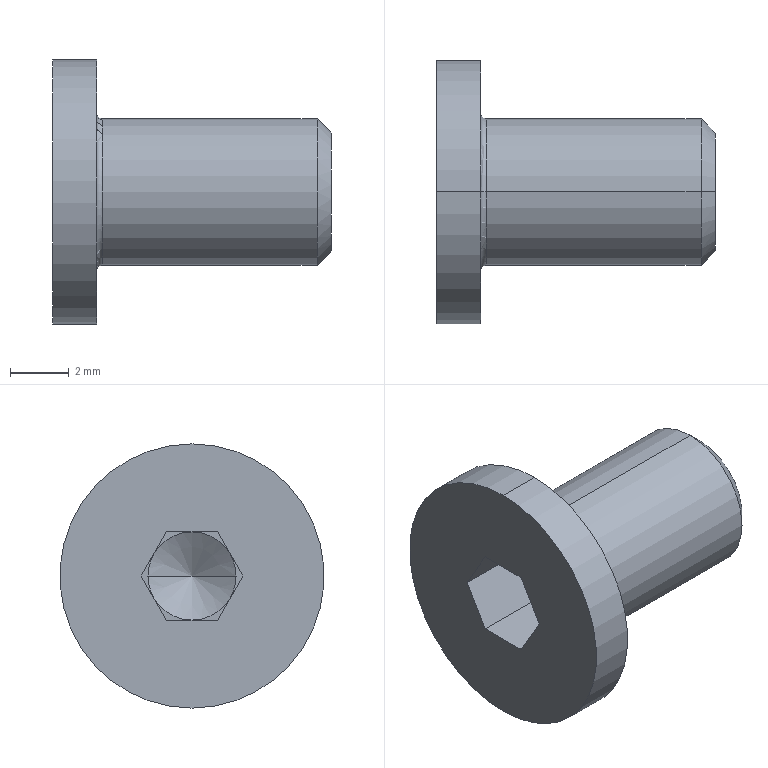Part | STEP file | CBSTS5-8-1 | 1 solid | 25 faces | box 9.5 x 9 x 9 mm | volume 225.454 mm3 | plane 15 | cone 4 | cylinder 4 | torus 2 | commonest cylinder face diameters 5 x2 9 x2
STEP:
#1=CARTESIAN_POINT('',(2.366,0.,0.));
#2=VERTEX_POINT('',#1);
#3=CARTESIAN_POINT('',(1.5,-1.5,0.));
#4=VERTEX_POINT('',#3);
#5=CARTESIAN_POINT('',(1.5,-1.5,0.));
#6=DIRECTION('',(-0.5,-0.866,0.));
#7=VECTOR('',#6,1000.);
#8=LINE('',#5,#7);
#9=EDGE_CURVE('',#2,#4,#8,.T.);
#10=ORIENTED_EDGE('',*,*,#9,.F.);
#11=CARTESIAN_POINT('',(1.5,1.5,0.));
#12=VERTEX_POINT('',#11);
#13=CARTESIAN_POINT('',(1.5,1.5,0.));
#14=DIRECTION('',(-0.5,0.866,0.));
#15=VECTOR('',#14,1000.);
#16=LINE('',#13,#15);
#17=EDGE_CURVE('',#2,#12,#16,.T.);
#18=ORIENTED_EDGE('',*,*,#17,.T.);
#19=CARTESIAN_POINT('',(1.5,1.299,-0.75));
#20=VERTEX_POINT('',#19);
#21=CARTESIAN_POINT('',(1.5,0.,0.));
#22=DIRECTION('',(1.,0.,0.));
#23=DIRECTION('',(0.,1.,0.));
#24=AXIS2_PLACEMENT_3D('',#21,#22,#23);
#25=CIRCLE('',#24,1.5);
#26=EDGE_CURVE('',#20,#12,#25,.T.);
#27=ORIENTED_EDGE('',*,*,#26,.F.);
#28=CARTESIAN_POINT('',(1.5,0.,-1.5));
#29=VERTEX_POINT('',#28);
#30=CARTESIAN_POINT('',(1.5,0.,0.));
#31=DIRECTION('',(1.,0.,0.));
#32=DIRECTION('',(0.,1.,0.));
#33=AXIS2_PLACEMENT_3D('',#30,#31,#32);
#34=CIRCLE('',#33,1.5);
#35=EDGE_CURVE('',#29,#20,#34,.T.);
#36=ORIENTED_EDGE('',*,*,#35,.F.);
#37=CARTESIAN_POINT('',(1.5,-1.299,-0.75));
#38=VERTEX_POINT('',#37);
#39=CARTESIAN_POINT('',(1.5,0.,0.));
#40=DIRECTION('',(1.,0.,0.));
#41=DIRECTION('',(0.,1.,0.));
#42=AXIS2_PLACEMENT_3D('',#39,#40,#41);
#43=CIRCLE('',#42,1.5);
#44=EDGE_CURVE('',#38,#29,#43,.T.);
#45=ORIENTED_EDGE('',*,*,#44,.F.);
#46=CARTESIAN_POINT('',(1.5,0.,0.));
#47=DIRECTION('',(1.,0.,0.));
#48=DIRECTION('',(0.,1.,0.));
#49=AXIS2_PLACEMENT_3D('',#46,#47,#48);
#50=CIRCLE('',#49,1.5);
#51=EDGE_CURVE('',#4,#38,#50,.T.);
#52=ORIENTED_EDGE('',*,*,#51,.F.);
#53=EDGE_LOOP('',(#10,#18,#27,#36,#45,#52));
#54=FACE_OUTER_BOUND('',#53,.T.);
#55=CARTESIAN_POINT('',(1.5,0.,0.));
#56=DIRECTION('',(-1.,0.,0.));
#57=DIRECTION('',(0.,-1.,0.));
#58=AXIS2_PLACEMENT_3D('',#55,#56,#57);
#59=CONICAL_SURFACE('',#58,1.5,1.047);
#60=ADVANCED_FACE('',(#54),#59,.F.);
#61=CARTESIAN_POINT('',(8.,0.,-2.01));
#62=VERTEX_POINT('',#61);
#63=CARTESIAN_POINT('',(8.,0.,2.01));
#64=VERTEX_POINT('',#63);
#65=CARTESIAN_POINT('',(8.,0.,0.));
#66=DIRECTION('',(1.,0.,0.));
#67=DIRECTION('',(0.,0.,-1.));
#68=AXIS2_PLACEMENT_3D('',#65,#66,#67);
#69=CIRCLE('',#68,2.01);
#70=EDGE_CURVE('',#62,#64,#69,.T.);
#71=ORIENTED_EDGE('',*,*,#70,.F.);
#72=CARTESIAN_POINT('',(7.51,0.,-2.5));
#73=VERTEX_POINT('',#72);
#74=CARTESIAN_POINT('',(7.51,0.,-2.5));
#75=DIRECTION('',(-0.7071,0.,-0.7071));
#76=VECTOR('',#75,1000.);
#77=LINE('',#74,#76);
#78=EDGE_CURVE('',#62,#73,#77,.T.);
#79=ORIENTED_EDGE('',*,*,#78,.T.);
#80=CARTESIAN_POINT('',(7.51,0.,2.5));
#81=VERTEX_POINT('',#80);
#82=CARTESIAN_POINT('',(7.51,0.,0.));
#83=DIRECTION('',(1.,0.,0.));
#84=DIRECTION('',(0.,0.,-1.));
#85=AXIS2_PLACEMENT_3D('',#82,#83,#84);
#86=CIRCLE('',#85,2.5);
#87=EDGE_CURVE('',#73,#81,#86,.T.);
#88=ORIENTED_EDGE('',*,*,#87,.T.);
#89=CARTESIAN_POINT('',(7.51,0.,2.5));
#90=DIRECTION('',(-0.7071,0.,0.7071));
#91=VECTOR('',#90,1000.);
#92=LINE('',#89,#91);
#93=EDGE_CURVE('',#64,#81,#92,.T.);
#94=ORIENTED_EDGE('',*,*,#93,.F.);
#95=EDGE_LOOP('',(#71,#79,#88,#94));
#96=FACE_OUTER_BOUND('',#95,.T.);
#97=CARTESIAN_POINT('',(7.51,0.,0.));
#98=DIRECTION('',(-1.,0.,0.));
#99=DIRECTION('',(0.,0.,1.));
#100=AXIS2_PLACEMENT_3D('',#97,#98,#99);
#101=CONICAL_SURFACE('',#100,2.5,0.7854);
#102=ADVANCED_FACE('',(#96),#101,.T.);
#103=CARTESIAN_POINT('',(0.2,0.,-2.5));
#104=VERTEX_POINT('',#103);
#105=CARTESIAN_POINT('',(0.2,0.,2.5));
#106=VERTEX_POINT('',#105);
#107=CARTESIAN_POINT('',(0.2,0.,0.));
#108=DIRECTION('',(1.,0.,0.));
#109=DIRECTION('',(0.,0.,-1.));
#110=AXIS2_PLACEMENT_3D('',#107,#108,#109);
#111=CIRCLE('',#110,2.5);
#112=EDGE_CURVE('',#104,#106,#111,.T.);
#113=ORIENTED_EDGE('',*,*,#112,.T.);
#114=CARTESIAN_POINT('',(8.,0.,2.5));
#115=DIRECTION('',(1.,0.,0.));
#116=VECTOR('',#115,1000.);
#117=LINE('',#114,#116);
#118=EDGE_CURVE('',#106,#81,#117,.T.);
#119=ORIENTED_EDGE('',*,*,#118,.T.);
#120=ORIENTED_EDGE('',*,*,#87,.F.);
#121=CARTESIAN_POINT('',(8.,0.,-2.5));
#122=DIRECTION('',(1.,0.,0.));
#123=VECTOR('',#122,1000.);
#124=LINE('',#121,#123);
#125=EDGE_CURVE('',#104,#73,#124,.T.);
#126=ORIENTED_EDGE('',*,*,#125,.F.);
#127=EDGE_LOOP('',(#113,#119,#120,#126));
#128=FACE_OUTER_BOUND('',#127,.T.);
#129=CARTESIAN_POINT('',(8.,0.,0.));
#130=DIRECTION('',(1.,0.,0.));
#131=DIRECTION('',(0.,0.,-1.));
#132=AXIS2_PLACEMENT_3D('',#129,#130,#131);
#133=CYLINDRICAL_SURFACE('',#132,2.5);
#134=ADVANCED_FACE('',(#128),#133,.T.);
#135=CARTESIAN_POINT('',(0.2,0.,0.));
#136=DIRECTION('',(1.,0.,0.));
#137=DIRECTION('',(0.,0.,-1.));
#138=AXIS2_PLACEMENT_3D('',#135,#136,#137);
#139=CIRCLE('',#138,2.5);
#140=EDGE_CURVE('',#106,#104,#139,.T.);
#141=ORIENTED_EDGE('',*,*,#140,.F.);
#142=CARTESIAN_POINT('',(0.,0.,2.7));
#143=VERTEX_POINT('',#142);
#144=CARTESIAN_POINT('',(0.2,0.,2.7));
#145=DIRECTION('',(0.,1.,0.));
#146=DIRECTION('',(0.,0.,1.));
#147=AXIS2_PLACEMENT_3D('',#144,#145,#146);
#148=CIRCLE('',#147,0.2);
#149=EDGE_CURVE('',#106,#143,#148,.T.);
#150=ORIENTED_EDGE('',*,*,#149,.T.);
#151=CARTESIAN_POINT('',(0.,0.,-2.7));
#152=VERTEX_POINT('',#151);
#153=CARTESIAN_POINT('',(0.,0.,0.));
#154=DIRECTION('',(1.,0.,0.));
#155=DIRECTION('',(0.,0.,-1.));
#156=AXIS2_PLACEMENT_3D('',#153,#154,#155);
#157=CIRCLE('',#156,2.7);
#158=EDGE_CURVE('',#143,#152,#157,.T.);
#159=ORIENTED_EDGE('',*,*,#158,.T.);
#160=CARTESIAN_POINT('',(0.2,0.,-2.7));
#161=DIRECTION('',(0.,-1.,0.));
#162=DIRECTION('',(0.,0.,-1.));
#163=AXIS2_PLACEMENT_3D('',#160,#161,#162);
#164=CIRCLE('',#163,0.2);
#165=EDGE_CURVE('',#104,#152,#164,.T.);
#166=ORIENTED_EDGE('',*,*,#165,.F.);
#167=EDGE_LOOP('',(#141,#150,#159,#166));
#168=FACE_OUTER_BOUND('',#167,.T.);
#169=CARTESIAN_POINT('',(0.2,0.,0.));
#170=DIRECTION('',(1.,0.,0.));
#171=DIRECTION('',(0.,0.,-1.));
#172=AXIS2_PLACEMENT_3D('',#169,#170,#171);
#173=TOROIDAL_SURFACE('',#172,2.7,0.2);
#174=ADVANCED_FACE('',(#168),#173,.F.);
#175=CARTESIAN_POINT('',(-1.5,0.,-4.5));
#176=VERTEX_POINT('',#175);
#177=CARTESIAN_POINT('',(-1.5,0.,4.5));
#178=VERTEX_POINT('',#177);
#179=CARTESIAN_POINT('',(-1.5,0.,0.));
#180=DIRECTION('',(1.,0.,0.));
#181=DIRECTION('',(0.,0.,-1.));
#182=AXIS2_PLACEMENT_3D('',#179,#180,#181);
#183=CIRCLE('',#182,4.5);
#184=EDGE_CURVE('',#176,#178,#183,.T.);
#185=ORIENTED_EDGE('',*,*,#184,.T.);
#186=CARTESIAN_POINT('',(0.,0.,4.5));
#187=VERTEX_POINT('',#186);
#188=CARTESIAN_POINT('',(8.,0.,4.5));
#189=DIRECTION('',(1.,0.,0.));
#190=VECTOR('',#189,1000.);
#191=LINE('',#188,#190);
#192=EDGE_CURVE('',#178,#187,#191,.T.);
#193=ORIENTED_EDGE('',*,*,#192,.T.);
#194=CARTESIAN_POINT('',(0.,0.,-4.5));
#195=VERTEX_POINT('',#194);
#196=CARTESIAN_POINT('',(0.,0.,0.));
#197=DIRECTION('',(1.,0.,0.));
#198=DIRECTION('',(0.,0.,-1.));
#199=AXIS2_PLACEMENT_3D('',#196,#197,#198);
#200=CIRCLE('',#199,4.5);
#201=EDGE_CURVE('',#195,#187,#200,.T.);
#202=ORIENTED_EDGE('',*,*,#201,.F.);
#203=CARTESIAN_POINT('',(8.,0.,-4.5));
#204=DIRECTION('',(1.,0.,0.));
#205=VECTOR('',#204,1000.);
#206=LINE('',#203,#205);
#207=EDGE_CURVE('',#176,#195,#206,.T.);
#208=ORIENTED_EDGE('',*,*,#207,.F.);
#209=EDGE_LOOP('',(#185,#193,#202,#208));
#210=FACE_OUTER_BOUND('',#209,.T.);
#211=CARTESIAN_POINT('',(8.,0.,0.));
#212=DIRECTION('',(1.,0.,0.));
#213=DIRECTION('',(0.,0.,-1.));
#214=AXIS2_PLACEMENT_3D('',#211,#212,#213);
#215=CYLINDRICAL_SURFACE('',#214,4.5);
#216=ADVANCED_FACE('',(#210),#215,.T.);
#217=ORIENTED_EDGE('',*,*,#184,.F.);
#218=CARTESIAN_POINT('',(-1.5,0.,0.));
#219=DIRECTION('',(1.,0.,0.));
#220=DIRECTION('',(0.,0.,-1.));
#221=AXIS2_PLACEMENT_3D('',#218,#219,#220);
#222=CIRCLE('',#221,4.5);
#223=EDGE_CURVE('',#178,#176,#222,.T.);
#224=ORIENTED_EDGE('',*,*,#223,.F.);
#225=EDGE_LOOP('',(#217,#224));
#226=FACE_OUTER_BOUND('',#225,.T.);
#227=CARTESIAN_POINT('',(-1.5,-1.732,0.));
#228=VERTEX_POINT('',#227);
#229=CARTESIAN_POINT('',(-1.5,-0.866,-1.5));
#230=VERTEX_POINT('',#229);
#231=CARTESIAN_POINT('',(-1.5,-1.732,0.));
#232=DIRECTION('',(0.,0.5,-0.866));
#233=VECTOR('',#232,1000.);
#234=LINE('',#231,#233);
#235=EDGE_CURVE('',#228,#230,#234,.T.);
#236=ORIENTED_EDGE('',*,*,#235,.T.);
#237=CARTESIAN_POINT('',(-1.5,0.866,-1.5));
#238=VERTEX_POINT('',#237);
#239=CARTESIAN_POINT('',(-1.5,-0.866,-1.5));
#240=DIRECTION('',(0.,1.,0.));
#241=VECTOR('',#240,1000.);
#242=LINE('',#239,#241);
#243=EDGE_CURVE('',#230,#238,#242,.T.);
#244=ORIENTED_EDGE('',*,*,#243,.T.);
#245=CARTESIAN_POINT('',(-1.5,1.732,0.));
#246=VERTEX_POINT('',#245);
#247=CARTESIAN_POINT('',(-1.5,0.866,-1.5));
#248=DIRECTION('',(0.,0.5,0.866));
#249=VECTOR('',#248,1000.);
#250=LINE('',#247,#249);
#251=EDGE_CURVE('',#238,#246,#250,.T.);
#252=ORIENTED_EDGE('',*,*,#251,.T.);
#253=CARTESIAN_POINT('',(-1.5,0.866,1.5));
#254=VERTEX_POINT('',#253);
#255=CARTESIAN_POINT('',(-1.5,1.732,0.));
#256=DIRECTION('',(0.,-0.5,0.866));
#257=VECTOR('',#256,1000.);
#258=LINE('',#255,#257);
#259=EDGE_CURVE('',#246,#254,#258,.T.);
#260=ORIENTED_EDGE('',*,*,#259,.T.);
#261=CARTESIAN_POINT('',(-1.5,-0.866,1.5));
#262=VERTEX_POINT('',#261);
#263=CARTESIAN_POINT('',(-1.5,0.866,1.5));
#264=DIRECTION('',(0.,-1.,0.));
#265=VECTOR('',#264,1000.);
#266=LINE('',#263,#265);
#267=EDGE_CURVE('',#254,#262,#266,.T.);
#268=ORIENTED_EDGE('',*,*,#267,.T.);
#269=CARTESIAN_POINT('',(-1.5,-0.866,1.5));
#270=DIRECTION('',(0.,-0.5,-0.866));
#271=VECTOR('',#270,1000.);
#272=LINE('',#269,#271);
#273=EDGE_CURVE('',#262,#228,#272,.T.);
#274=ORIENTED_EDGE('',*,*,#273,.T.);
#275=EDGE_LOOP('',(#236,#244,#252,#260,#268,#274));
#276=FACE_BOUND('',#275,.T.);
#277=CARTESIAN_POINT('',(-1.5,0.,0.));
#278=DIRECTION('',(1.,0.,0.));
#279=DIRECTION('',(0.,0.,-1.));
#280=AXIS2_PLACEMENT_3D('',#277,#278,#279);
#281=PLANE('',#280);
#282=ADVANCED_FACE('',(#226,#276),#281,.F.);
#283=ORIENTED_EDGE('',*,*,#192,.F.);
#284=ORIENTED_EDGE('',*,*,#223,.T.);
#285=ORIENTED_EDGE('',*,*,#207,.T.);
#286=CARTESIAN_POINT('',(0.,0.,0.));
#287=DIRECTION('',(1.,0.,0.));
#288=DIRECTION('',(0.,0.,-1.));
#289=AXIS2_PLACEMENT_3D('',#286,#287,#288);
#290=CIRCLE('',#289,4.5);
#291=EDGE_CURVE('',#187,#195,#290,.T.);
#292=ORIENTED_EDGE('',*,*,#291,.F.);
#293=EDGE_LOOP('',(#283,#284,#285,#292));
#294=FACE_OUTER_BOUND('',#293,.T.);
#295=CARTESIAN_POINT('',(8.,0.,0.));
#296=DIRECTION('',(1.,0.,0.));
#297=DIRECTION('',(0.,0.,-1.));
#298=AXIS2_PLACEMENT_3D('',#295,#296,#297);
#299=CYLINDRICAL_SURFACE('',#298,4.5);
#300=ADVANCED_FACE('',(#294),#299,.T.);
#301=CARTESIAN_POINT('',(0.,0.,0.));
#302=DIRECTION('',(1.,0.,0.));
#303=DIRECTION('',(0.,0.,-1.));
#304=AXIS2_PLACEMENT_3D('',#301,#302,#303);
#305=CIRCLE('',#304,2.7);
#306=EDGE_CURVE('',#152,#143,#305,.T.);
#307=ORIENTED_EDGE('',*,*,#306,.F.);
#308=ORIENTED_EDGE('',*,*,#158,.F.);
#309=EDGE_LOOP('',(#307,#308));
#310=FACE_BOUND('',#309,.T.);
#311=ORIENTED_EDGE('',*,*,#201,.T.);
#312=ORIENTED_EDGE('',*,*,#291,.T.);
#313=EDGE_LOOP('',(#311,#312));
#314=FACE_OUTER_BOUND('',#313,.T.);
#315=CARTESIAN_POINT('',(0.,4.5,0.));
#316=DIRECTION('',(-1.,0.,0.));
#317=DIRECTION('',(0.,0.,1.));
#318=AXIS2_PLACEMENT_3D('',#315,#316,#317);
#319=PLANE('',#318);
#320=ADVANCED_FACE('',(#310,#314),#319,.F.);
#321=ORIENTED_EDGE('',*,*,#149,.F.);
#322=ORIENTED_EDGE('',*,*,#112,.F.);
#323=ORIENTED_EDGE('',*,*,#165,.T.);
#324=ORIENTED_EDGE('',*,*,#306,.T.);
#325=EDGE_LOOP('',(#321,#322,#323,#324));
#326=FACE_OUTER_BOUND('',#325,.T.);
#327=CARTESIAN_POINT('',(0.2,0.,0.));
#328=DIRECTION('',(1.,0.,0.));
#329=DIRECTION('',(0.,0.,-1.));
#330=AXIS2_PLACEMENT_3D('',#327,#328,#329);
#331=TOROIDAL_SURFACE('',#330,2.7,0.2);
#332=ADVANCED_FACE('',(#326),#331,.F.);
#333=ORIENTED_EDGE('',*,*,#118,.F.);
#334=ORIENTED_EDGE('',*,*,#140,.T.);
#335=ORIENTED_EDGE('',*,*,#125,.T.);
#336=CARTESIAN_POINT('',(7.51,0.,0.));
#337=DIRECTION('',(1.,0.,0.));
#338=DIRECTION('',(0.,0.,-1.));
#339=AXIS2_PLACEMENT_3D('',#336,#337,#338);
#340=CIRCLE('',#339,2.5);
#341=EDGE_CURVE('',#81,#73,#340,.T.);
#342=ORIENTED_EDGE('',*,*,#341,.F.);
#343=EDGE_LOOP('',(#333,#334,#335,#342));
#344=FACE_OUTER_BOUND('',#343,.T.);
#345=CARTESIAN_POINT('',(8.,0.,0.));
#346=DIRECTION('',(1.,0.,0.));
#347=DIRECTION('',(0.,0.,-1.));
#348=AXIS2_PLACEMENT_3D('',#345,#346,#347);
#349=CYLINDRICAL_SURFACE('',#348,2.5);
#350=ADVANCED_FACE('',(#344),#349,.T.);
#351=ORIENTED_EDGE('',*,*,#78,.F.);
#352=CARTESIAN_POINT('',(8.,0.,0.));
#353=DIRECTION('',(1.,0.,0.));
#354=DIRECTION('',(0.,0.,-1.));
#355=AXIS2_PLACEMENT_3D('',#352,#353,#354);
#356=CIRCLE('',#355,2.01);
#357=EDGE_CURVE('',#64,#62,#356,.T.);
#358=ORIENTED_EDGE('',*,*,#357,.F.);
#359=ORIENTED_EDGE('',*,*,#93,.T.);
#360=ORIENTED_EDGE('',*,*,#341,.T.);
#361=EDGE_LOOP('',(#351,#358,#359,#360));
#362=FACE_OUTER_BOUND('',#361,.T.);
#363=CARTESIAN_POINT('',(7.51,0.,0.));
#364=DIRECTION('',(-1.,0.,0.));
#365=DIRECTION('',(0.,0.,1.));
#366=AXIS2_PLACEMENT_3D('',#363,#364,#365);
#367=CONICAL_SURFACE('',#366,2.5,0.7854);
#368=ADVANCED_FACE('',(#362),#367,.T.);
#369=ORIENTED_EDGE('',*,*,#357,.T.);
#370=ORIENTED_EDGE('',*,*,#70,.T.);
#371=EDGE_LOOP('',(#369,#370));
#372=FACE_OUTER_BOUND('',#371,.T.);
#373=CARTESIAN_POINT('',(8.,2.01,0.));
#374=DIRECTION('',(-1.,0.,0.));
#375=DIRECTION('',(0.,0.,1.));
#376=AXIS2_PLACEMENT_3D('',#373,#374,#375);
#377=PLANE('',#376);
#378=ADVANCED_FACE('',(#372),#377,.F.);
#379=ORIENTED_EDGE('',*,*,#267,.F.);
#380=CARTESIAN_POINT('',(1.5,0.866,1.5));
#381=VERTEX_POINT('',#380);
#382=CARTESIAN_POINT('',(1.5,0.866,1.5));
#383=DIRECTION('',(-1.,0.,0.));
#384=VECTOR('',#383,1000.);
#385=LINE('',#382,#384);
#386=EDGE_CURVE('',#381,#254,#385,.T.);
#387=ORIENTED_EDGE('',*,*,#386,.F.);
#388=CARTESIAN_POINT('',(1.5,0.,1.5));
#389=VERTEX_POINT('',#388);
#390=CARTESIAN_POINT('',(1.5,0.866,1.5));
#391=DIRECTION('',(0.,-1.,0.));
#392=VECTOR('',#391,1000.);
#393=LINE('',#390,#392);
#394=EDGE_CURVE('',#381,#389,#393,.T.);
#395=ORIENTED_EDGE('',*,*,#394,.T.);
#396=CARTESIAN_POINT('',(1.5,-0.866,1.5));
#397=VERTEX_POINT('',#396);
#398=CARTESIAN_POINT('',(1.5,0.866,1.5));
#399=DIRECTION('',(0.,-1.,0.));
#400=VECTOR('',#399,1000.);
#401=LINE('',#398,#400);
#402=EDGE_CURVE('',#389,#397,#401,.T.);
#403=ORIENTED_EDGE('',*,*,#402,.T.);
#404=CARTESIAN_POINT('',(1.5,-0.866,1.5));
#405=DIRECTION('',(-1.,0.,0.));
#406=VECTOR('',#405,1000.);
#407=LINE('',#404,#406);
#408=EDGE_CURVE('',#397,#262,#407,.T.);
#409=ORIENTED_EDGE('',*,*,#408,.T.);
#410=EDGE_LOOP('',(#379,#387,#395,#403,#409));
#411=FACE_OUTER_BOUND('',#410,.T.);
#412=CARTESIAN_POINT('',(1.5,0.866,1.5));
#413=DIRECTION('',(0.,0.,-1.));
#414=DIRECTION('',(-1.,0.,0.));
#415=AXIS2_PLACEMENT_3D('',#412,#413,#414);
#416=PLANE('',#415);
#417=ADVANCED_FACE('',(#411),#416,.T.);
#418=ORIENTED_EDGE('',*,*,#273,.F.);
#419=ORIENTED_EDGE('',*,*,#408,.F.);
#420=CARTESIAN_POINT('',(1.5,-1.299,0.75));
#421=VERTEX_POINT('',#420);
#422=CARTESIAN_POINT('',(1.5,-0.866,1.5));
#423=DIRECTION('',(0.,-0.5,-0.866));
#424=VECTOR('',#423,1000.);
#425=LINE('',#422,#424);
#426=EDGE_CURVE('',#397,#421,#425,.T.);
#427=ORIENTED_EDGE('',*,*,#426,.T.);
#428=CARTESIAN_POINT('',(1.5,-1.732,0.));
#429=VERTEX_POINT('',#428);
#430=CARTESIAN_POINT('',(1.5,-0.866,1.5));
#431=DIRECTION('',(0.,-0.5,-0.866));
#432=VECTOR('',#431,1000.);
#433=LINE('',#430,#432);
#434=EDGE_CURVE('',#421,#429,#433,.T.);
#435=ORIENTED_EDGE('',*,*,#434,.T.);
#436=CARTESIAN_POINT('',(1.5,-1.732,0.));
#437=DIRECTION('',(-1.,0.,0.));
#438=VECTOR('',#437,1000.);
#439=LINE('',#436,#438);
#440=EDGE_CURVE('',#429,#228,#439,.T.);
#441=ORIENTED_EDGE('',*,*,#440,.T.);
#442=EDGE_LOOP('',(#418,#419,#427,#435,#441));
#443=FACE_OUTER_BOUND('',#442,.T.);
#444=CARTESIAN_POINT('',(1.5,-0.866,1.5));
#445=DIRECTION('',(0.,0.866,-0.5));
#446=DIRECTION('',(0.,0.5,0.866));
#447=AXIS2_PLACEMENT_3D('',#444,#445,#446);
#448=PLANE('',#447);
#449=ADVANCED_FACE('',(#443),#448,.T.);
#450=ORIENTED_EDGE('',*,*,#235,.F.);
#451=ORIENTED_EDGE('',*,*,#440,.F.);
#452=CARTESIAN_POINT('',(1.5,-1.732,0.));
#453=DIRECTION('',(0.,0.5,-0.866));
#454=VECTOR('',#453,1000.);
#455=LINE('',#452,#454);
#456=EDGE_CURVE('',#429,#38,#455,.T.);
#457=ORIENTED_EDGE('',*,*,#456,.T.);
#458=CARTESIAN_POINT('',(1.5,-0.866,-1.5));
#459=VERTEX_POINT('',#458);
#460=CARTESIAN_POINT('',(1.5,-1.732,0.));
#461=DIRECTION('',(0.,0.5,-0.866));
#462=VECTOR('',#461,1000.);
#463=LINE('',#460,#462);
#464=EDGE_CURVE('',#38,#459,#463,.T.);
#465=ORIENTED_EDGE('',*,*,#464,.T.);
#466=CARTESIAN_POINT('',(1.5,-0.866,-1.5));
#467=DIRECTION('',(-1.,0.,0.));
#468=VECTOR('',#467,1000.);
#469=LINE('',#466,#468);
#470=EDGE_CURVE('',#459,#230,#469,.T.);
#471=ORIENTED_EDGE('',*,*,#470,.T.);
#472=EDGE_LOOP('',(#450,#451,#457,#465,#471));
#473=FACE_OUTER_BOUND('',#472,.T.);
#474=CARTESIAN_POINT('',(1.5,-1.732,0.));
#475=DIRECTION('',(0.,0.866,0.5));
#476=DIRECTION('',(0.,-0.5,0.866));
#477=AXIS2_PLACEMENT_3D('',#474,#475,#476);
#478=PLANE('',#477);
#479=ADVANCED_FACE('',(#473),#478,.T.);
#480=ORIENTED_EDGE('',*,*,#243,.F.);
#481=ORIENTED_EDGE('',*,*,#470,.F.);
#482=CARTESIAN_POINT('',(1.5,-0.866,-1.5));
#483=DIRECTION('',(0.,1.,0.));
#484=VECTOR('',#483,1000.);
#485=LINE('',#482,#484);
#486=EDGE_CURVE('',#459,#29,#485,.T.);
#487=ORIENTED_EDGE('',*,*,#486,.T.);
#488=CARTESIAN_POINT('',(1.5,0.866,-1.5));
#489=VERTEX_POINT('',#488);
#490=CARTESIAN_POINT('',(1.5,-0.866,-1.5));
#491=DIRECTION('',(0.,1.,0.));
#492=VECTOR('',#491,1000.);
#493=LINE('',#490,#492);
#494=EDGE_CURVE('',#29,#489,#493,.T.);
#495=ORIENTED_EDGE('',*,*,#494,.T.);
#496=CARTESIAN_POINT('',(1.5,0.866,-1.5));
#497=DIRECTION('',(-1.,0.,0.));
#498=VECTOR('',#497,1000.);
#499=LINE('',#496,#498);
#500=EDGE_CURVE('',#489,#238,#499,.T.);
#501=ORIENTED_EDGE('',*,*,#500,.T.);
#502=EDGE_LOOP('',(#480,#481,#487,#495,#501));
#503=FACE_OUTER_BOUND('',#502,.T.);
#504=CARTESIAN_POINT('',(1.5,-0.866,-1.5));
#505=DIRECTION('',(0.,0.,1.));
#506=DIRECTION('',(1.,0.,0.));
#507=AXIS2_PLACEMENT_3D('',#504,#505,#506);
#508=PLANE('',#507);
#509=ADVANCED_FACE('',(#503),#508,.T.);
#510=ORIENTED_EDGE('',*,*,#251,.F.);
#511=ORIENTED_EDGE('',*,*,#500,.F.);
#512=CARTESIAN_POINT('',(1.5,0.866,-1.5));
#513=DIRECTION('',(0.,0.5,0.866));
#514=VECTOR('',#513,1000.);
#515=LINE('',#512,#514);
#516=EDGE_CURVE('',#489,#20,#515,.T.);
#517=ORIENTED_EDGE('',*,*,#516,.T.);
#518=CARTESIAN_POINT('',(1.5,1.732,0.));
#519=VERTEX_POINT('',#518);
#520=CARTESIAN_POINT('',(1.5,0.866,-1.5));
#521=DIRECTION('',(0.,0.5,0.866));
#522=VECTOR('',#521,1000.);
#523=LINE('',#520,#522);
#524=EDGE_CURVE('',#20,#519,#523,.T.);
#525=ORIENTED_EDGE('',*,*,#524,.T.);
#526=CARTESIAN_POINT('',(1.5,1.732,0.));
#527=DIRECTION('',(-1.,0.,0.));
#528=VECTOR('',#527,1000.);
#529=LINE('',#526,#528);
#530=EDGE_CURVE('',#519,#246,#529,.T.);
#531=ORIENTED_EDGE('',*,*,#530,.T.);
#532=EDGE_LOOP('',(#510,#511,#517,#525,#531));
#533=FACE_OUTER_BOUND('',#532,.T.);
#534=CARTESIAN_POINT('',(1.5,0.866,-1.5));
#535=DIRECTION('',(0.,-0.866,0.5));
#536=DIRECTION('',(0.,-0.5,-0.866));
#537=AXIS2_PLACEMENT_3D('',#534,#535,#536);
#538=PLANE('',#537);
#539=ADVANCED_FACE('',(#533),#538,.T.);
#540=ORIENTED_EDGE('',*,*,#259,.F.);
#541=ORIENTED_EDGE('',*,*,#530,.F.);
#542=CARTESIAN_POINT('',(1.5,1.299,0.75));
#543=VERTEX_POINT('',#542);
#544=CARTESIAN_POINT('',(1.5,1.732,0.));
#545=DIRECTION('',(0.,-0.5,0.866));
#546=VECTOR('',#545,1000.);
#547=LINE('',#544,#546);
#548=EDGE_CURVE('',#519,#543,#547,.T.);
#549=ORIENTED_EDGE('',*,*,#548,.T.);
#550=CARTESIAN_POINT('',(1.5,1.732,0.));
#551=DIRECTION('',(0.,-0.5,0.866));
#552=VECTOR('',#551,1000.);
#553=LINE('',#550,#552);
#554=EDGE_CURVE('',#543,#381,#553,.T.);
#555=ORIENTED_EDGE('',*,*,#554,.T.);
#556=ORIENTED_EDGE('',*,*,#386,.T.);
#557=EDGE_LOOP('',(#540,#541,#549,#555,#556));
#558=FACE_OUTER_BOUND('',#557,.T.);
#559=CARTESIAN_POINT('',(1.5,1.732,0.));
#560=DIRECTION('',(0.,-0.866,-0.5));
#561=DIRECTION('',(0.,0.5,-0.866));
#562=AXIS2_PLACEMENT_3D('',#559,#560,#561);
#563=PLANE('',#562);
#564=ADVANCED_FACE('',(#558),#563,.T.);
#565=ORIENTED_EDGE('',*,*,#35,.T.);
#566=ORIENTED_EDGE('',*,*,#516,.F.);
#567=ORIENTED_EDGE('',*,*,#494,.F.);
#568=EDGE_LOOP('',(#565,#566,#567));
#569=FACE_OUTER_BOUND('',#568,.T.);
#570=CARTESIAN_POINT('',(1.5,0.,0.));
#571=DIRECTION('',(1.,0.,0.));
#572=DIRECTION('',(0.,0.,-1.));
#573=AXIS2_PLACEMENT_3D('',#570,#571,#572);
#574=PLANE('',#573);
#575=ADVANCED_FACE('',(#569),#574,.F.);
#576=ORIENTED_EDGE('',*,*,#524,.F.);
#577=ORIENTED_EDGE('',*,*,#26,.T.);
#578=CARTESIAN_POINT('',(1.5,0.,0.));
#579=DIRECTION('',(1.,0.,0.));
#580=DIRECTION('',(0.,1.,0.));
#581=AXIS2_PLACEMENT_3D('',#578,#579,#580);
#582=CIRCLE('',#581,1.5);
#583=EDGE_CURVE('',#12,#543,#582,.T.);
#584=ORIENTED_EDGE('',*,*,#583,.T.);
#585=ORIENTED_EDGE('',*,*,#548,.F.);
#586=EDGE_LOOP('',(#576,#577,#584,#585));
#587=FACE_OUTER_BOUND('',#586,.T.);
#588=CARTESIAN_POINT('',(1.5,0.,0.));
#589=DIRECTION('',(1.,0.,0.));
#590=DIRECTION('',(0.,0.,-1.));
#591=AXIS2_PLACEMENT_3D('',#588,#589,#590);
#592=PLANE('',#591);
#593=ADVANCED_FACE('',(#587),#592,.F.);
#594=CARTESIAN_POINT('',(1.5,0.,0.));
#595=DIRECTION('',(1.,0.,0.));
#596=DIRECTION('',(0.,1.,0.));
#597=AXIS2_PLACEMENT_3D('',#594,#595,#596);
#598=CIRCLE('',#597,1.5);
#599=EDGE_CURVE('',#543,#389,#598,.T.);
#600=ORIENTED_EDGE('',*,*,#599,.T.);
#601=ORIENTED_EDGE('',*,*,#394,.F.);
#602=ORIENTED_EDGE('',*,*,#554,.F.);
#603=EDGE_LOOP('',(#600,#601,#602));
#604=FACE_OUTER_BOUND('',#603,.T.);
#605=CARTESIAN_POINT('',(1.5,0.,0.));
#606=DIRECTION('',(1.,0.,0.));
#607=DIRECTION('',(0.,0.,-1.));
#608=AXIS2_PLACEMENT_3D('',#605,#606,#607);
#609=PLANE('',#608);
#610=ADVANCED_FACE('',(#604),#609,.F.);
#611=CARTESIAN_POINT('',(1.5,0.,0.));
#612=DIRECTION('',(1.,0.,0.));
#613=DIRECTION('',(0.,1.,0.));
#614=AXIS2_PLACEMENT_3D('',#611,#612,#613);
#615=CIRCLE('',#614,1.5);
#616=EDGE_CURVE('',#389,#421,#615,.T.);
#617=ORIENTED_EDGE('',*,*,#616,.T.);
#618=ORIENTED_EDGE('',*,*,#426,.F.);
#619=ORIENTED_EDGE('',*,*,#402,.F.);
#620=EDGE_LOOP('',(#617,#618,#619));
#621=FACE_OUTER_BOUND('',#620,.T.);
#622=CARTESIAN_POINT('',(1.5,0.,0.));
#623=DIRECTION('',(1.,0.,0.));
#624=DIRECTION('',(0.,0.,-1.));
#625=AXIS2_PLACEMENT_3D('',#622,#623,#624);
#626=PLANE('',#625);
#627=ADVANCED_FACE('',(#621),#626,.F.);
#628=CARTESIAN_POINT('',(1.5,0.,0.));
#629=DIRECTION('',(1.,0.,0.));
#630=DIRECTION('',(0.,1.,0.));
#631=AXIS2_PLACEMENT_3D('',#628,#629,#630);
#632=CIRCLE('',#631,1.5);
#633=EDGE_CURVE('',#421,#4,#632,.T.);
#634=ORIENTED_EDGE('',*,*,#633,.T.);
#635=ORIENTED_EDGE('',*,*,#51,.T.);
#636=ORIENTED_EDGE('',*,*,#456,.F.);
#637=ORIENTED_EDGE('',*,*,#434,.F.);
#638=EDGE_LOOP('',(#634,#635,#636,#637));
#639=FACE_OUTER_BOUND('',#638,.T.);
#640=CARTESIAN_POINT('',(1.5,0.,0.));
#641=DIRECTION('',(1.,0.,0.));
#642=DIRECTION('',(0.,0.,-1.));
#643=AXIS2_PLACEMENT_3D('',#640,#641,#642);
#644=PLANE('',#643);
#645=ADVANCED_FACE('',(#639),#644,.F.);
#646=ORIENTED_EDGE('',*,*,#44,.T.);
#647=ORIENTED_EDGE('',*,*,#486,.F.);
#648=ORIENTED_EDGE('',*,*,#464,.F.);
#649=EDGE_LOOP('',(#646,#647,#648));
#650=FACE_OUTER_BOUND('',#649,.T.);
#651=CARTESIAN_POINT('',(1.5,0.,0.));
#652=DIRECTION('',(1.,0.,0.));
#653=DIRECTION('',(0.,0.,-1.));
#654=AXIS2_PLACEMENT_3D('',#651,#652,#653);
#655=PLANE('',#654);
#656=ADVANCED_FACE('',(#650),#655,.F.);
#657=ORIENTED_EDGE('',*,*,#17,.F.);
#658=ORIENTED_EDGE('',*,*,#9,.T.);
#659=ORIENTED_EDGE('',*,*,#633,.F.);
#660=ORIENTED_EDGE('',*,*,#616,.F.);
#661=ORIENTED_EDGE('',*,*,#599,.F.);
#662=ORIENTED_EDGE('',*,*,#583,.F.);
#663=EDGE_LOOP('',(#657,#658,#659,#660,#661,#662));
#664=FACE_OUTER_BOUND('',#663,.T.);
#665=CARTESIAN_POINT('',(1.5,0.,0.));
#666=DIRECTION('',(-1.,0.,0.));
#667=DIRECTION('',(0.,-1.,0.));
#668=AXIS2_PLACEMENT_3D('',#665,#666,#667);
#669=CONICAL_SURFACE('',#668,1.5,1.047);
#670=ADVANCED_FACE('',(#664),#669,.F.);
#671=CLOSED_SHELL('',(#60,#102,#134,#174,#216,#282,#300,#320,#332,#350,#368,#378,#417,#449,#479,#509,#539,#564,#575,#593,#610,#627,#645,#656,#670));
#672=MANIFOLD_SOLID_BREP('',#671);
#673=CARTESIAN_POINT('',(0.,0.,0.));
#674=DIRECTION('',(0.,0.,1.));
#675=DIRECTION('',(1.,0.,0.));
#676=AXIS2_PLACEMENT_3D('',#673,#674,#675);
#677=(LENGTH_UNIT()NAMED_UNIT(*)SI_UNIT(.MILLI.,.METRE.));
#678=UNCERTAINTY_MEASURE_WITH_UNIT(LENGTH_MEASURE(0.00001),#677,'','');
#679=(NAMED_UNIT(*)PLANE_ANGLE_UNIT()SI_UNIT($,.RADIAN.));
#680=(NAMED_UNIT(*)SI_UNIT($,.STERADIAN.)SOLID_ANGLE_UNIT());
#681=(GEOMETRIC_REPRESENTATION_CONTEXT(3)GLOBAL_UNCERTAINTY_ASSIGNED_CONTEXT((#678))GLOBAL_UNIT_ASSIGNED_CONTEXT((#677,#679,#680))REPRESENTATION_CONTEXT('',''));
#682=ADVANCED_BREP_SHAPE_REPRESENTATION('',(#672,#676),#681);